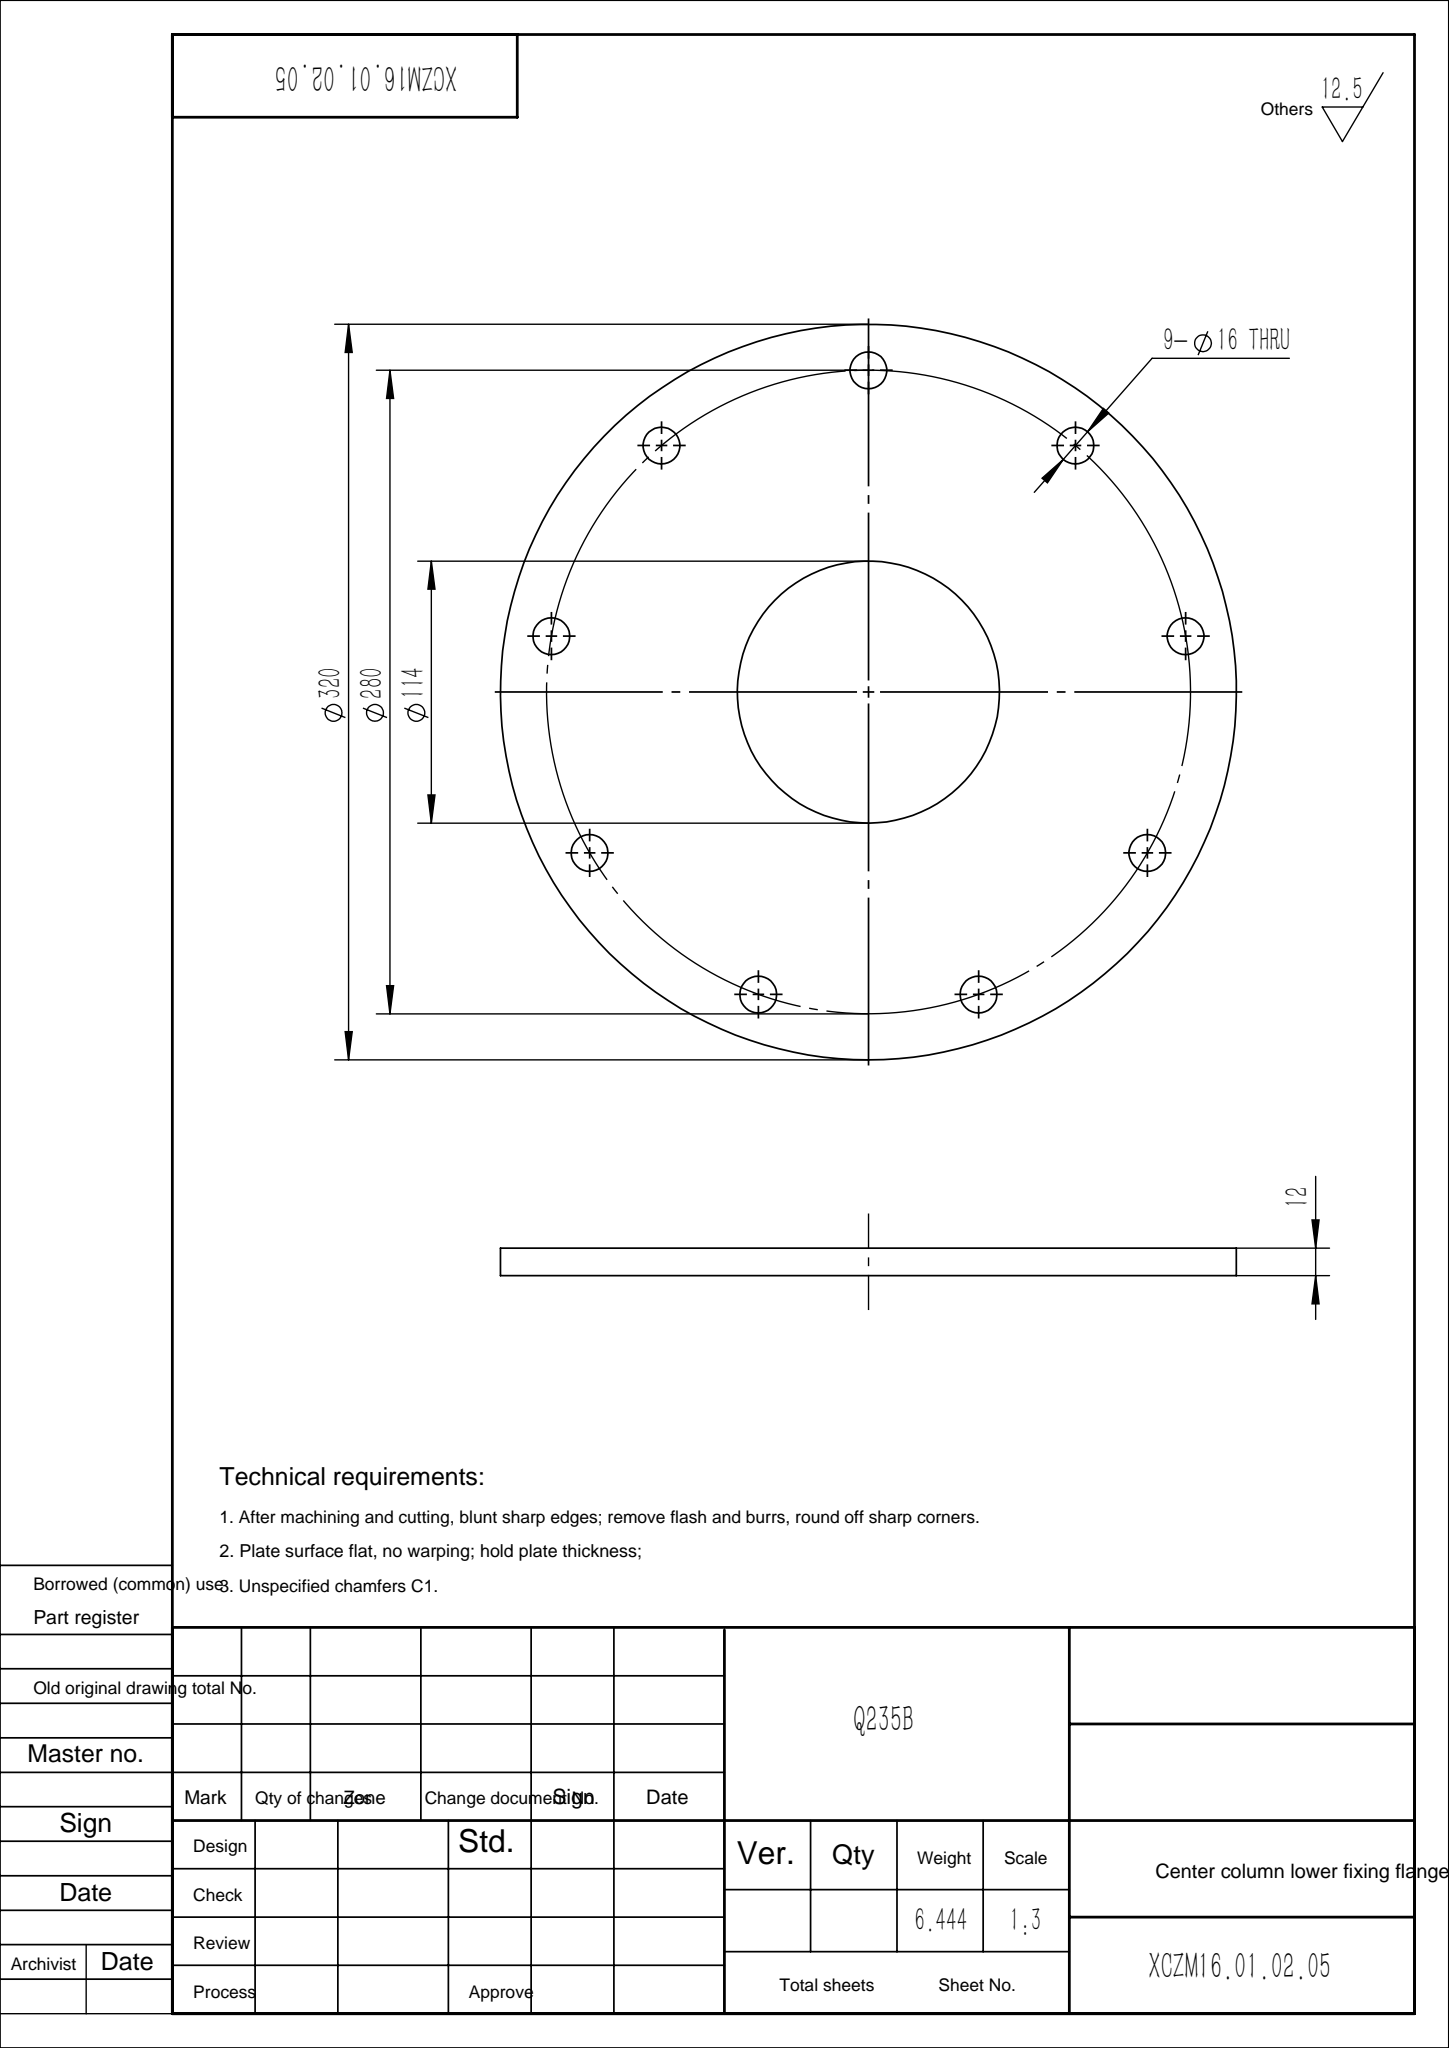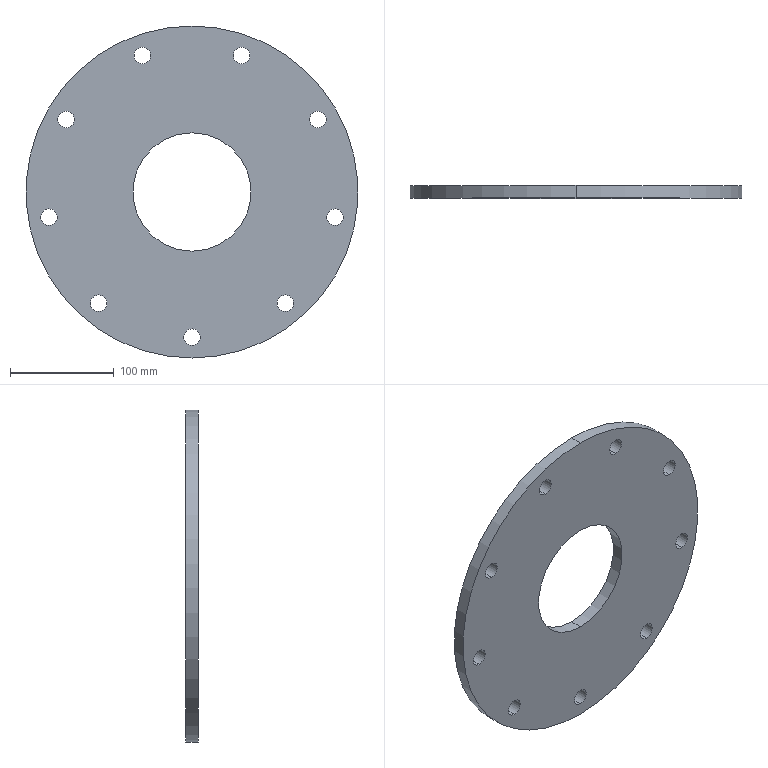Part | SolidWorks | features Extrusion 1 | 1 solid | 24 faces | box 320 x 12 x 320 mm | volume 820898 mm3 | cylinder 22 | plane 2 | commonest cylinder face diameters 16 x18 114 x2 320 x2
STEP:
#1=CARTESIAN_POINT('',(-89.99,12.,-115.246));
#2=VERTEX_POINT('',#1);
#3=CARTESIAN_POINT('',(-89.99,12.,-99.246));
#4=VERTEX_POINT('',#3);
#5=CARTESIAN_POINT('',(-89.99,12.,-107.246));
#6=DIRECTION('',(0.,1.,0.));
#7=DIRECTION('',(0.,0.,1.));
#8=AXIS2_PLACEMENT_3D('',#5,#6,#7);
#9=CIRCLE('',#8,8.);
#10=EDGE_CURVE('',#2,#4,#9,.T.);
#11=ORIENTED_EDGE('',*,*,#10,.T.);
#12=CARTESIAN_POINT('',(-89.99,0.,-99.246));
#13=VERTEX_POINT('',#12);
#14=CARTESIAN_POINT('',(-89.99,12.,-99.246));
#15=DIRECTION('',(0.,-1.,0.));
#16=VECTOR('',#15,1000.);
#17=LINE('',#14,#16);
#18=EDGE_CURVE('',#4,#13,#17,.T.);
#19=ORIENTED_EDGE('',*,*,#18,.T.);
#20=CARTESIAN_POINT('',(-89.99,0.,-115.246));
#21=VERTEX_POINT('',#20);
#22=CARTESIAN_POINT('',(-89.99,0.,-107.246));
#23=DIRECTION('',(0.,1.,0.));
#24=DIRECTION('',(0.,0.,1.));
#25=AXIS2_PLACEMENT_3D('',#22,#23,#24);
#26=CIRCLE('',#25,8.);
#27=EDGE_CURVE('',#21,#13,#26,.T.);
#28=ORIENTED_EDGE('',*,*,#27,.F.);
#29=CARTESIAN_POINT('',(-89.99,12.,-115.246));
#30=DIRECTION('',(0.,-1.,0.));
#31=VECTOR('',#30,1000.);
#32=LINE('',#29,#31);
#33=EDGE_CURVE('',#2,#21,#32,.T.);
#34=ORIENTED_EDGE('',*,*,#33,.F.);
#35=EDGE_LOOP('',(#11,#19,#28,#34));
#36=FACE_OUTER_BOUND('',#35,.T.);
#37=CARTESIAN_POINT('',(-89.99,12.,-107.246));
#38=DIRECTION('',(0.,-1.,0.));
#39=DIRECTION('',(0.,0.,-1.));
#40=AXIS2_PLACEMENT_3D('',#37,#38,#39);
#41=CYLINDRICAL_SURFACE('',#40,8.);
#42=ADVANCED_FACE('',(#36),#41,.F.);
#43=CARTESIAN_POINT('',(-137.873,12.,-32.311));
#44=VERTEX_POINT('',#43);
#45=CARTESIAN_POINT('',(-137.873,12.,-16.311));
#46=VERTEX_POINT('',#45);
#47=CARTESIAN_POINT('',(-137.873,12.,-24.311));
#48=DIRECTION('',(0.,1.,0.));
#49=DIRECTION('',(0.,0.,1.));
#50=AXIS2_PLACEMENT_3D('',#47,#48,#49);
#51=CIRCLE('',#50,8.);
#52=EDGE_CURVE('',#44,#46,#51,.T.);
#53=ORIENTED_EDGE('',*,*,#52,.T.);
#54=CARTESIAN_POINT('',(-137.873,0.,-16.311));
#55=VERTEX_POINT('',#54);
#56=CARTESIAN_POINT('',(-137.873,12.,-16.311));
#57=DIRECTION('',(0.,-1.,0.));
#58=VECTOR('',#57,1000.);
#59=LINE('',#56,#58);
#60=EDGE_CURVE('',#46,#55,#59,.T.);
#61=ORIENTED_EDGE('',*,*,#60,.T.);
#62=CARTESIAN_POINT('',(-137.873,0.,-32.311));
#63=VERTEX_POINT('',#62);
#64=CARTESIAN_POINT('',(-137.873,0.,-24.311));
#65=DIRECTION('',(0.,1.,0.));
#66=DIRECTION('',(0.,0.,1.));
#67=AXIS2_PLACEMENT_3D('',#64,#65,#66);
#68=CIRCLE('',#67,8.);
#69=EDGE_CURVE('',#63,#55,#68,.T.);
#70=ORIENTED_EDGE('',*,*,#69,.F.);
#71=CARTESIAN_POINT('',(-137.873,12.,-32.311));
#72=DIRECTION('',(0.,-1.,0.));
#73=VECTOR('',#72,1000.);
#74=LINE('',#71,#73);
#75=EDGE_CURVE('',#44,#63,#74,.T.);
#76=ORIENTED_EDGE('',*,*,#75,.F.);
#77=EDGE_LOOP('',(#53,#61,#70,#76));
#78=FACE_OUTER_BOUND('',#77,.T.);
#79=CARTESIAN_POINT('',(-137.873,12.,-24.311));
#80=DIRECTION('',(0.,-1.,0.));
#81=DIRECTION('',(0.,0.,-1.));
#82=AXIS2_PLACEMENT_3D('',#79,#80,#81);
#83=CYLINDRICAL_SURFACE('',#82,8.);
#84=ADVANCED_FACE('',(#78),#83,.F.);
#85=CARTESIAN_POINT('',(-121.244,12.,62.));
#86=VERTEX_POINT('',#85);
#87=CARTESIAN_POINT('',(-121.244,12.,78.));
#88=VERTEX_POINT('',#87);
#89=CARTESIAN_POINT('',(-121.244,12.,70.));
#90=DIRECTION('',(0.,1.,0.));
#91=DIRECTION('',(0.,0.,1.));
#92=AXIS2_PLACEMENT_3D('',#89,#90,#91);
#93=CIRCLE('',#92,8.);
#94=EDGE_CURVE('',#86,#88,#93,.T.);
#95=ORIENTED_EDGE('',*,*,#94,.T.);
#96=CARTESIAN_POINT('',(-121.244,0.,78.));
#97=VERTEX_POINT('',#96);
#98=CARTESIAN_POINT('',(-121.244,12.,78.));
#99=DIRECTION('',(0.,-1.,0.));
#100=VECTOR('',#99,1000.);
#101=LINE('',#98,#100);
#102=EDGE_CURVE('',#88,#97,#101,.T.);
#103=ORIENTED_EDGE('',*,*,#102,.T.);
#104=CARTESIAN_POINT('',(-121.244,0.,62.));
#105=VERTEX_POINT('',#104);
#106=CARTESIAN_POINT('',(-121.244,0.,70.));
#107=DIRECTION('',(0.,1.,0.));
#108=DIRECTION('',(0.,0.,1.));
#109=AXIS2_PLACEMENT_3D('',#106,#107,#108);
#110=CIRCLE('',#109,8.);
#111=EDGE_CURVE('',#105,#97,#110,.T.);
#112=ORIENTED_EDGE('',*,*,#111,.F.);
#113=CARTESIAN_POINT('',(-121.244,12.,62.));
#114=DIRECTION('',(0.,-1.,0.));
#115=VECTOR('',#114,1000.);
#116=LINE('',#113,#115);
#117=EDGE_CURVE('',#86,#105,#116,.T.);
#118=ORIENTED_EDGE('',*,*,#117,.F.);
#119=EDGE_LOOP('',(#95,#103,#112,#118));
#120=FACE_OUTER_BOUND('',#119,.T.);
#121=CARTESIAN_POINT('',(-121.244,12.,70.));
#122=DIRECTION('',(0.,-1.,0.));
#123=DIRECTION('',(0.,0.,-1.));
#124=AXIS2_PLACEMENT_3D('',#121,#122,#123);
#125=CYLINDRICAL_SURFACE('',#124,8.);
#126=ADVANCED_FACE('',(#120),#125,.F.);
#127=CARTESIAN_POINT('',(-47.883,12.,123.557));
#128=VERTEX_POINT('',#127);
#129=CARTESIAN_POINT('',(-47.883,12.,139.557));
#130=VERTEX_POINT('',#129);
#131=CARTESIAN_POINT('',(-47.883,12.,131.557));
#132=DIRECTION('',(0.,1.,0.));
#133=DIRECTION('',(0.,0.,1.));
#134=AXIS2_PLACEMENT_3D('',#131,#132,#133);
#135=CIRCLE('',#134,8.);
#136=EDGE_CURVE('',#128,#130,#135,.T.);
#137=ORIENTED_EDGE('',*,*,#136,.T.);
#138=CARTESIAN_POINT('',(-47.883,0.,139.557));
#139=VERTEX_POINT('',#138);
#140=CARTESIAN_POINT('',(-47.883,12.,139.557));
#141=DIRECTION('',(0.,-1.,0.));
#142=VECTOR('',#141,1000.);
#143=LINE('',#140,#142);
#144=EDGE_CURVE('',#130,#139,#143,.T.);
#145=ORIENTED_EDGE('',*,*,#144,.T.);
#146=CARTESIAN_POINT('',(-47.883,0.,123.557));
#147=VERTEX_POINT('',#146);
#148=CARTESIAN_POINT('',(-47.883,0.,131.557));
#149=DIRECTION('',(0.,1.,0.));
#150=DIRECTION('',(0.,0.,1.));
#151=AXIS2_PLACEMENT_3D('',#148,#149,#150);
#152=CIRCLE('',#151,8.);
#153=EDGE_CURVE('',#147,#139,#152,.T.);
#154=ORIENTED_EDGE('',*,*,#153,.F.);
#155=CARTESIAN_POINT('',(-47.883,12.,123.557));
#156=DIRECTION('',(0.,-1.,0.));
#157=VECTOR('',#156,1000.);
#158=LINE('',#155,#157);
#159=EDGE_CURVE('',#128,#147,#158,.T.);
#160=ORIENTED_EDGE('',*,*,#159,.F.);
#161=EDGE_LOOP('',(#137,#145,#154,#160));
#162=FACE_OUTER_BOUND('',#161,.T.);
#163=CARTESIAN_POINT('',(-47.883,12.,131.557));
#164=DIRECTION('',(0.,-1.,0.));
#165=DIRECTION('',(0.,0.,-1.));
#166=AXIS2_PLACEMENT_3D('',#163,#164,#165);
#167=CYLINDRICAL_SURFACE('',#166,8.);
#168=ADVANCED_FACE('',(#162),#167,.F.);
#169=CARTESIAN_POINT('',(47.883,12.,123.557));
#170=VERTEX_POINT('',#169);
#171=CARTESIAN_POINT('',(47.883,12.,139.557));
#172=VERTEX_POINT('',#171);
#173=CARTESIAN_POINT('',(47.883,12.,131.557));
#174=DIRECTION('',(0.,1.,0.));
#175=DIRECTION('',(0.,0.,1.));
#176=AXIS2_PLACEMENT_3D('',#173,#174,#175);
#177=CIRCLE('',#176,8.);
#178=EDGE_CURVE('',#170,#172,#177,.T.);
#179=ORIENTED_EDGE('',*,*,#178,.T.);
#180=CARTESIAN_POINT('',(47.883,0.,139.557));
#181=VERTEX_POINT('',#180);
#182=CARTESIAN_POINT('',(47.883,12.,139.557));
#183=DIRECTION('',(0.,-1.,0.));
#184=VECTOR('',#183,1000.);
#185=LINE('',#182,#184);
#186=EDGE_CURVE('',#172,#181,#185,.T.);
#187=ORIENTED_EDGE('',*,*,#186,.T.);
#188=CARTESIAN_POINT('',(47.883,0.,123.557));
#189=VERTEX_POINT('',#188);
#190=CARTESIAN_POINT('',(47.883,0.,131.557));
#191=DIRECTION('',(0.,1.,0.));
#192=DIRECTION('',(0.,0.,1.));
#193=AXIS2_PLACEMENT_3D('',#190,#191,#192);
#194=CIRCLE('',#193,8.);
#195=EDGE_CURVE('',#189,#181,#194,.T.);
#196=ORIENTED_EDGE('',*,*,#195,.F.);
#197=CARTESIAN_POINT('',(47.883,12.,123.557));
#198=DIRECTION('',(0.,-1.,0.));
#199=VECTOR('',#198,1000.);
#200=LINE('',#197,#199);
#201=EDGE_CURVE('',#170,#189,#200,.T.);
#202=ORIENTED_EDGE('',*,*,#201,.F.);
#203=EDGE_LOOP('',(#179,#187,#196,#202));
#204=FACE_OUTER_BOUND('',#203,.T.);
#205=CARTESIAN_POINT('',(47.883,12.,131.557));
#206=DIRECTION('',(0.,-1.,0.));
#207=DIRECTION('',(0.,0.,-1.));
#208=AXIS2_PLACEMENT_3D('',#205,#206,#207);
#209=CYLINDRICAL_SURFACE('',#208,8.);
#210=ADVANCED_FACE('',(#204),#209,.F.);
#211=CARTESIAN_POINT('',(121.244,12.,62.));
#212=VERTEX_POINT('',#211);
#213=CARTESIAN_POINT('',(121.244,12.,78.));
#214=VERTEX_POINT('',#213);
#215=CARTESIAN_POINT('',(121.244,12.,70.));
#216=DIRECTION('',(0.,1.,0.));
#217=DIRECTION('',(0.,0.,1.));
#218=AXIS2_PLACEMENT_3D('',#215,#216,#217);
#219=CIRCLE('',#218,8.);
#220=EDGE_CURVE('',#212,#214,#219,.T.);
#221=ORIENTED_EDGE('',*,*,#220,.T.);
#222=CARTESIAN_POINT('',(121.244,0.,78.));
#223=VERTEX_POINT('',#222);
#224=CARTESIAN_POINT('',(121.244,12.,78.));
#225=DIRECTION('',(0.,-1.,0.));
#226=VECTOR('',#225,1000.);
#227=LINE('',#224,#226);
#228=EDGE_CURVE('',#214,#223,#227,.T.);
#229=ORIENTED_EDGE('',*,*,#228,.T.);
#230=CARTESIAN_POINT('',(121.244,0.,62.));
#231=VERTEX_POINT('',#230);
#232=CARTESIAN_POINT('',(121.244,0.,70.));
#233=DIRECTION('',(0.,1.,0.));
#234=DIRECTION('',(0.,0.,1.));
#235=AXIS2_PLACEMENT_3D('',#232,#233,#234);
#236=CIRCLE('',#235,8.);
#237=EDGE_CURVE('',#231,#223,#236,.T.);
#238=ORIENTED_EDGE('',*,*,#237,.F.);
#239=CARTESIAN_POINT('',(121.244,12.,62.));
#240=DIRECTION('',(0.,-1.,0.));
#241=VECTOR('',#240,1000.);
#242=LINE('',#239,#241);
#243=EDGE_CURVE('',#212,#231,#242,.T.);
#244=ORIENTED_EDGE('',*,*,#243,.F.);
#245=EDGE_LOOP('',(#221,#229,#238,#244));
#246=FACE_OUTER_BOUND('',#245,.T.);
#247=CARTESIAN_POINT('',(121.244,12.,70.));
#248=DIRECTION('',(0.,-1.,0.));
#249=DIRECTION('',(0.,0.,-1.));
#250=AXIS2_PLACEMENT_3D('',#247,#248,#249);
#251=CYLINDRICAL_SURFACE('',#250,8.);
#252=ADVANCED_FACE('',(#246),#251,.F.);
#253=CARTESIAN_POINT('',(137.873,12.,-32.311));
#254=VERTEX_POINT('',#253);
#255=CARTESIAN_POINT('',(137.873,12.,-16.311));
#256=VERTEX_POINT('',#255);
#257=CARTESIAN_POINT('',(137.873,12.,-24.311));
#258=DIRECTION('',(0.,1.,0.));
#259=DIRECTION('',(0.,0.,1.));
#260=AXIS2_PLACEMENT_3D('',#257,#258,#259);
#261=CIRCLE('',#260,8.);
#262=EDGE_CURVE('',#254,#256,#261,.T.);
#263=ORIENTED_EDGE('',*,*,#262,.T.);
#264=CARTESIAN_POINT('',(137.873,0.,-16.311));
#265=VERTEX_POINT('',#264);
#266=CARTESIAN_POINT('',(137.873,12.,-16.311));
#267=DIRECTION('',(0.,-1.,0.));
#268=VECTOR('',#267,1000.);
#269=LINE('',#266,#268);
#270=EDGE_CURVE('',#256,#265,#269,.T.);
#271=ORIENTED_EDGE('',*,*,#270,.T.);
#272=CARTESIAN_POINT('',(137.873,0.,-32.311));
#273=VERTEX_POINT('',#272);
#274=CARTESIAN_POINT('',(137.873,0.,-24.311));
#275=DIRECTION('',(0.,1.,0.));
#276=DIRECTION('',(0.,0.,1.));
#277=AXIS2_PLACEMENT_3D('',#274,#275,#276);
#278=CIRCLE('',#277,8.);
#279=EDGE_CURVE('',#273,#265,#278,.T.);
#280=ORIENTED_EDGE('',*,*,#279,.F.);
#281=CARTESIAN_POINT('',(137.873,12.,-32.311));
#282=DIRECTION('',(0.,-1.,0.));
#283=VECTOR('',#282,1000.);
#284=LINE('',#281,#283);
#285=EDGE_CURVE('',#254,#273,#284,.T.);
#286=ORIENTED_EDGE('',*,*,#285,.F.);
#287=EDGE_LOOP('',(#263,#271,#280,#286));
#288=FACE_OUTER_BOUND('',#287,.T.);
#289=CARTESIAN_POINT('',(137.873,12.,-24.311));
#290=DIRECTION('',(0.,-1.,0.));
#291=DIRECTION('',(0.,0.,-1.));
#292=AXIS2_PLACEMENT_3D('',#289,#290,#291);
#293=CYLINDRICAL_SURFACE('',#292,8.);
#294=ADVANCED_FACE('',(#288),#293,.F.);
#295=CARTESIAN_POINT('',(89.99,12.,-115.246));
#296=VERTEX_POINT('',#295);
#297=CARTESIAN_POINT('',(89.99,12.,-99.246));
#298=VERTEX_POINT('',#297);
#299=CARTESIAN_POINT('',(89.99,12.,-107.246));
#300=DIRECTION('',(0.,1.,0.));
#301=DIRECTION('',(0.,0.,1.));
#302=AXIS2_PLACEMENT_3D('',#299,#300,#301);
#303=CIRCLE('',#302,8.);
#304=EDGE_CURVE('',#296,#298,#303,.T.);
#305=ORIENTED_EDGE('',*,*,#304,.T.);
#306=CARTESIAN_POINT('',(89.99,0.,-99.246));
#307=VERTEX_POINT('',#306);
#308=CARTESIAN_POINT('',(89.99,12.,-99.246));
#309=DIRECTION('',(0.,-1.,0.));
#310=VECTOR('',#309,1000.);
#311=LINE('',#308,#310);
#312=EDGE_CURVE('',#298,#307,#311,.T.);
#313=ORIENTED_EDGE('',*,*,#312,.T.);
#314=CARTESIAN_POINT('',(89.99,0.,-115.246));
#315=VERTEX_POINT('',#314);
#316=CARTESIAN_POINT('',(89.99,0.,-107.246));
#317=DIRECTION('',(0.,1.,0.));
#318=DIRECTION('',(0.,0.,1.));
#319=AXIS2_PLACEMENT_3D('',#316,#317,#318);
#320=CIRCLE('',#319,8.);
#321=EDGE_CURVE('',#315,#307,#320,.T.);
#322=ORIENTED_EDGE('',*,*,#321,.F.);
#323=CARTESIAN_POINT('',(89.99,12.,-115.246));
#324=DIRECTION('',(0.,-1.,0.));
#325=VECTOR('',#324,1000.);
#326=LINE('',#323,#325);
#327=EDGE_CURVE('',#296,#315,#326,.T.);
#328=ORIENTED_EDGE('',*,*,#327,.F.);
#329=EDGE_LOOP('',(#305,#313,#322,#328));
#330=FACE_OUTER_BOUND('',#329,.T.);
#331=CARTESIAN_POINT('',(89.99,12.,-107.246));
#332=DIRECTION('',(0.,-1.,0.));
#333=DIRECTION('',(0.,0.,-1.));
#334=AXIS2_PLACEMENT_3D('',#331,#332,#333);
#335=CYLINDRICAL_SURFACE('',#334,8.);
#336=ADVANCED_FACE('',(#330),#335,.F.);
#337=CARTESIAN_POINT('',(0.,12.,-148.));
#338=VERTEX_POINT('',#337);
#339=CARTESIAN_POINT('',(0.,12.,-132.));
#340=VERTEX_POINT('',#339);
#341=CARTESIAN_POINT('',(0.,12.,-140.));
#342=DIRECTION('',(0.,1.,0.));
#343=DIRECTION('',(0.,0.,1.));
#344=AXIS2_PLACEMENT_3D('',#341,#342,#343);
#345=CIRCLE('',#344,8.);
#346=EDGE_CURVE('',#338,#340,#345,.T.);
#347=ORIENTED_EDGE('',*,*,#346,.T.);
#348=CARTESIAN_POINT('',(0.,0.,-132.));
#349=VERTEX_POINT('',#348);
#350=CARTESIAN_POINT('',(0.,12.,-132.));
#351=DIRECTION('',(0.,-1.,0.));
#352=VECTOR('',#351,1000.);
#353=LINE('',#350,#352);
#354=EDGE_CURVE('',#340,#349,#353,.T.);
#355=ORIENTED_EDGE('',*,*,#354,.T.);
#356=CARTESIAN_POINT('',(0.,0.,-148.));
#357=VERTEX_POINT('',#356);
#358=CARTESIAN_POINT('',(0.,0.,-140.));
#359=DIRECTION('',(0.,1.,0.));
#360=DIRECTION('',(0.,0.,1.));
#361=AXIS2_PLACEMENT_3D('',#358,#359,#360);
#362=CIRCLE('',#361,8.);
#363=EDGE_CURVE('',#357,#349,#362,.T.);
#364=ORIENTED_EDGE('',*,*,#363,.F.);
#365=CARTESIAN_POINT('',(0.,12.,-148.));
#366=DIRECTION('',(0.,-1.,0.));
#367=VECTOR('',#366,1000.);
#368=LINE('',#365,#367);
#369=EDGE_CURVE('',#338,#357,#368,.T.);
#370=ORIENTED_EDGE('',*,*,#369,.F.);
#371=EDGE_LOOP('',(#347,#355,#364,#370));
#372=FACE_OUTER_BOUND('',#371,.T.);
#373=CARTESIAN_POINT('',(0.,12.,-140.));
#374=DIRECTION('',(0.,-1.,0.));
#375=DIRECTION('',(0.,0.,-1.));
#376=AXIS2_PLACEMENT_3D('',#373,#374,#375);
#377=CYLINDRICAL_SURFACE('',#376,8.);
#378=ADVANCED_FACE('',(#372),#377,.F.);
#379=CARTESIAN_POINT('',(0.,12.,-57.));
#380=VERTEX_POINT('',#379);
#381=CARTESIAN_POINT('',(0.,12.,57.));
#382=VERTEX_POINT('',#381);
#383=CARTESIAN_POINT('',(0.,12.,0.));
#384=DIRECTION('',(0.,1.,0.));
#385=DIRECTION('',(0.,0.,1.));
#386=AXIS2_PLACEMENT_3D('',#383,#384,#385);
#387=CIRCLE('',#386,57.);
#388=EDGE_CURVE('',#380,#382,#387,.T.);
#389=ORIENTED_EDGE('',*,*,#388,.T.);
#390=CARTESIAN_POINT('',(0.,0.,57.));
#391=VERTEX_POINT('',#390);
#392=CARTESIAN_POINT('',(0.,12.,57.));
#393=DIRECTION('',(0.,-1.,0.));
#394=VECTOR('',#393,1000.);
#395=LINE('',#392,#394);
#396=EDGE_CURVE('',#382,#391,#395,.T.);
#397=ORIENTED_EDGE('',*,*,#396,.T.);
#398=CARTESIAN_POINT('',(0.,0.,-57.));
#399=VERTEX_POINT('',#398);
#400=CARTESIAN_POINT('',(0.,0.,0.));
#401=DIRECTION('',(0.,1.,0.));
#402=DIRECTION('',(0.,0.,1.));
#403=AXIS2_PLACEMENT_3D('',#400,#401,#402);
#404=CIRCLE('',#403,57.);
#405=EDGE_CURVE('',#399,#391,#404,.T.);
#406=ORIENTED_EDGE('',*,*,#405,.F.);
#407=CARTESIAN_POINT('',(0.,12.,-57.));
#408=DIRECTION('',(0.,-1.,0.));
#409=VECTOR('',#408,1000.);
#410=LINE('',#407,#409);
#411=EDGE_CURVE('',#380,#399,#410,.T.);
#412=ORIENTED_EDGE('',*,*,#411,.F.);
#413=EDGE_LOOP('',(#389,#397,#406,#412));
#414=FACE_OUTER_BOUND('',#413,.T.);
#415=CARTESIAN_POINT('',(0.,12.,0.));
#416=DIRECTION('',(0.,-1.,0.));
#417=DIRECTION('',(0.,0.,-1.));
#418=AXIS2_PLACEMENT_3D('',#415,#416,#417);
#419=CYLINDRICAL_SURFACE('',#418,57.);
#420=ADVANCED_FACE('',(#414),#419,.F.);
#421=CARTESIAN_POINT('',(0.,12.,160.));
#422=VERTEX_POINT('',#421);
#423=CARTESIAN_POINT('',(0.,12.,-160.));
#424=VERTEX_POINT('',#423);
#425=CARTESIAN_POINT('',(0.,12.,0.));
#426=DIRECTION('',(0.,1.,0.));
#427=DIRECTION('',(0.,0.,1.));
#428=AXIS2_PLACEMENT_3D('',#425,#426,#427);
#429=CIRCLE('',#428,160.);
#430=EDGE_CURVE('',#422,#424,#429,.T.);
#431=ORIENTED_EDGE('',*,*,#430,.F.);
#432=CARTESIAN_POINT('',(0.,0.,160.));
#433=VERTEX_POINT('',#432);
#434=CARTESIAN_POINT('',(0.,12.,160.));
#435=DIRECTION('',(0.,-1.,0.));
#436=VECTOR('',#435,1000.);
#437=LINE('',#434,#436);
#438=EDGE_CURVE('',#422,#433,#437,.T.);
#439=ORIENTED_EDGE('',*,*,#438,.T.);
#440=CARTESIAN_POINT('',(0.,0.,-160.));
#441=VERTEX_POINT('',#440);
#442=CARTESIAN_POINT('',(0.,0.,0.));
#443=DIRECTION('',(0.,1.,0.));
#444=DIRECTION('',(0.,0.,1.));
#445=AXIS2_PLACEMENT_3D('',#442,#443,#444);
#446=CIRCLE('',#445,160.);
#447=EDGE_CURVE('',#433,#441,#446,.T.);
#448=ORIENTED_EDGE('',*,*,#447,.T.);
#449=CARTESIAN_POINT('',(0.,12.,-160.));
#450=DIRECTION('',(0.,-1.,0.));
#451=VECTOR('',#450,1000.);
#452=LINE('',#449,#451);
#453=EDGE_CURVE('',#424,#441,#452,.T.);
#454=ORIENTED_EDGE('',*,*,#453,.F.);
#455=EDGE_LOOP('',(#431,#439,#448,#454));
#456=FACE_OUTER_BOUND('',#455,.T.);
#457=CARTESIAN_POINT('',(0.,12.,0.));
#458=DIRECTION('',(0.,-1.,0.));
#459=DIRECTION('',(0.,0.,-1.));
#460=AXIS2_PLACEMENT_3D('',#457,#458,#459);
#461=CYLINDRICAL_SURFACE('',#460,160.);
#462=ADVANCED_FACE('',(#456),#461,.T.);
#463=ORIENTED_EDGE('',*,*,#52,.F.);
#464=CARTESIAN_POINT('',(-137.873,12.,-24.311));
#465=DIRECTION('',(0.,1.,0.));
#466=DIRECTION('',(0.,0.,1.));
#467=AXIS2_PLACEMENT_3D('',#464,#465,#466);
#468=CIRCLE('',#467,8.);
#469=EDGE_CURVE('',#46,#44,#468,.T.);
#470=ORIENTED_EDGE('',*,*,#469,.F.);
#471=EDGE_LOOP('',(#463,#470));
#472=FACE_BOUND('',#471,.T.);
#473=ORIENTED_EDGE('',*,*,#136,.F.);
#474=CARTESIAN_POINT('',(-47.883,12.,131.557));
#475=DIRECTION('',(0.,1.,0.));
#476=DIRECTION('',(0.,0.,1.));
#477=AXIS2_PLACEMENT_3D('',#474,#475,#476);
#478=CIRCLE('',#477,8.);
#479=EDGE_CURVE('',#130,#128,#478,.T.);
#480=ORIENTED_EDGE('',*,*,#479,.F.);
#481=EDGE_LOOP('',(#473,#480));
#482=FACE_BOUND('',#481,.T.);
#483=ORIENTED_EDGE('',*,*,#220,.F.);
#484=CARTESIAN_POINT('',(121.244,12.,70.));
#485=DIRECTION('',(0.,1.,0.));
#486=DIRECTION('',(0.,0.,1.));
#487=AXIS2_PLACEMENT_3D('',#484,#485,#486);
#488=CIRCLE('',#487,8.);
#489=EDGE_CURVE('',#214,#212,#488,.T.);
#490=ORIENTED_EDGE('',*,*,#489,.F.);
#491=EDGE_LOOP('',(#483,#490));
#492=FACE_BOUND('',#491,.T.);
#493=ORIENTED_EDGE('',*,*,#304,.F.);
#494=CARTESIAN_POINT('',(89.99,12.,-107.246));
#495=DIRECTION('',(0.,1.,0.));
#496=DIRECTION('',(0.,0.,1.));
#497=AXIS2_PLACEMENT_3D('',#494,#495,#496);
#498=CIRCLE('',#497,8.);
#499=EDGE_CURVE('',#298,#296,#498,.T.);
#500=ORIENTED_EDGE('',*,*,#499,.F.);
#501=EDGE_LOOP('',(#493,#500));
#502=FACE_BOUND('',#501,.T.);
#503=ORIENTED_EDGE('',*,*,#388,.F.);
#504=CARTESIAN_POINT('',(0.,12.,0.));
#505=DIRECTION('',(0.,1.,0.));
#506=DIRECTION('',(0.,0.,1.));
#507=AXIS2_PLACEMENT_3D('',#504,#505,#506);
#508=CIRCLE('',#507,57.);
#509=EDGE_CURVE('',#382,#380,#508,.T.);
#510=ORIENTED_EDGE('',*,*,#509,.F.);
#511=EDGE_LOOP('',(#503,#510));
#512=FACE_BOUND('',#511,.T.);
#513=CARTESIAN_POINT('',(0.,12.,0.));
#514=DIRECTION('',(0.,1.,0.));
#515=DIRECTION('',(0.,0.,1.));
#516=AXIS2_PLACEMENT_3D('',#513,#514,#515);
#517=CIRCLE('',#516,160.);
#518=EDGE_CURVE('',#424,#422,#517,.T.);
#519=ORIENTED_EDGE('',*,*,#518,.T.);
#520=ORIENTED_EDGE('',*,*,#430,.T.);
#521=EDGE_LOOP('',(#519,#520));
#522=FACE_OUTER_BOUND('',#521,.T.);
#523=ORIENTED_EDGE('',*,*,#346,.F.);
#524=CARTESIAN_POINT('',(0.,12.,-140.));
#525=DIRECTION('',(0.,1.,0.));
#526=DIRECTION('',(0.,0.,1.));
#527=AXIS2_PLACEMENT_3D('',#524,#525,#526);
#528=CIRCLE('',#527,8.);
#529=EDGE_CURVE('',#340,#338,#528,.T.);
#530=ORIENTED_EDGE('',*,*,#529,.F.);
#531=EDGE_LOOP('',(#523,#530));
#532=FACE_BOUND('',#531,.T.);
#533=ORIENTED_EDGE('',*,*,#262,.F.);
#534=CARTESIAN_POINT('',(137.873,12.,-24.311));
#535=DIRECTION('',(0.,1.,0.));
#536=DIRECTION('',(0.,0.,1.));
#537=AXIS2_PLACEMENT_3D('',#534,#535,#536);
#538=CIRCLE('',#537,8.);
#539=EDGE_CURVE('',#256,#254,#538,.T.);
#540=ORIENTED_EDGE('',*,*,#539,.F.);
#541=EDGE_LOOP('',(#533,#540));
#542=FACE_BOUND('',#541,.T.);
#543=ORIENTED_EDGE('',*,*,#178,.F.);
#544=CARTESIAN_POINT('',(47.883,12.,131.557));
#545=DIRECTION('',(0.,1.,0.));
#546=DIRECTION('',(0.,0.,1.));
#547=AXIS2_PLACEMENT_3D('',#544,#545,#546);
#548=CIRCLE('',#547,8.);
#549=EDGE_CURVE('',#172,#170,#548,.T.);
#550=ORIENTED_EDGE('',*,*,#549,.F.);
#551=EDGE_LOOP('',(#543,#550));
#552=FACE_BOUND('',#551,.T.);
#553=ORIENTED_EDGE('',*,*,#94,.F.);
#554=CARTESIAN_POINT('',(-121.244,12.,70.));
#555=DIRECTION('',(0.,1.,0.));
#556=DIRECTION('',(0.,0.,1.));
#557=AXIS2_PLACEMENT_3D('',#554,#555,#556);
#558=CIRCLE('',#557,8.);
#559=EDGE_CURVE('',#88,#86,#558,.T.);
#560=ORIENTED_EDGE('',*,*,#559,.F.);
#561=EDGE_LOOP('',(#553,#560));
#562=FACE_BOUND('',#561,.T.);
#563=ORIENTED_EDGE('',*,*,#10,.F.);
#564=CARTESIAN_POINT('',(-89.99,12.,-107.246));
#565=DIRECTION('',(0.,1.,0.));
#566=DIRECTION('',(0.,0.,1.));
#567=AXIS2_PLACEMENT_3D('',#564,#565,#566);
#568=CIRCLE('',#567,8.);
#569=EDGE_CURVE('',#4,#2,#568,.T.);
#570=ORIENTED_EDGE('',*,*,#569,.F.);
#571=EDGE_LOOP('',(#563,#570));
#572=FACE_BOUND('',#571,.T.);
#573=CARTESIAN_POINT('',(0.,12.,0.));
#574=DIRECTION('',(0.,1.,0.));
#575=DIRECTION('',(0.,0.,1.));
#576=AXIS2_PLACEMENT_3D('',#573,#574,#575);
#577=PLANE('',#576);
#578=ADVANCED_FACE('',(#472,#482,#492,#502,#512,#522,#532,#542,#552,#562,#572),#577,.T.);
#579=CARTESIAN_POINT('',(0.,0.,0.));
#580=DIRECTION('',(0.,1.,0.));
#581=DIRECTION('',(0.,0.,1.));
#582=AXIS2_PLACEMENT_3D('',#579,#580,#581);
#583=CIRCLE('',#582,160.);
#584=EDGE_CURVE('',#441,#433,#583,.T.);
#585=ORIENTED_EDGE('',*,*,#584,.F.);
#586=ORIENTED_EDGE('',*,*,#447,.F.);
#587=EDGE_LOOP('',(#585,#586));
#588=FACE_OUTER_BOUND('',#587,.T.);
#589=ORIENTED_EDGE('',*,*,#405,.T.);
#590=CARTESIAN_POINT('',(0.,0.,0.));
#591=DIRECTION('',(0.,1.,0.));
#592=DIRECTION('',(0.,0.,1.));
#593=AXIS2_PLACEMENT_3D('',#590,#591,#592);
#594=CIRCLE('',#593,57.);
#595=EDGE_CURVE('',#391,#399,#594,.T.);
#596=ORIENTED_EDGE('',*,*,#595,.T.);
#597=EDGE_LOOP('',(#589,#596));
#598=FACE_BOUND('',#597,.T.);
#599=ORIENTED_EDGE('',*,*,#363,.T.);
#600=CARTESIAN_POINT('',(0.,0.,-140.));
#601=DIRECTION('',(0.,1.,0.));
#602=DIRECTION('',(0.,0.,1.));
#603=AXIS2_PLACEMENT_3D('',#600,#601,#602);
#604=CIRCLE('',#603,8.);
#605=EDGE_CURVE('',#349,#357,#604,.T.);
#606=ORIENTED_EDGE('',*,*,#605,.T.);
#607=EDGE_LOOP('',(#599,#606));
#608=FACE_BOUND('',#607,.T.);
#609=ORIENTED_EDGE('',*,*,#321,.T.);
#610=CARTESIAN_POINT('',(89.99,0.,-107.246));
#611=DIRECTION('',(0.,1.,0.));
#612=DIRECTION('',(0.,0.,1.));
#613=AXIS2_PLACEMENT_3D('',#610,#611,#612);
#614=CIRCLE('',#613,8.);
#615=EDGE_CURVE('',#307,#315,#614,.T.);
#616=ORIENTED_EDGE('',*,*,#615,.T.);
#617=EDGE_LOOP('',(#609,#616));
#618=FACE_BOUND('',#617,.T.);
#619=ORIENTED_EDGE('',*,*,#279,.T.);
#620=CARTESIAN_POINT('',(137.873,0.,-24.311));
#621=DIRECTION('',(0.,1.,0.));
#622=DIRECTION('',(0.,0.,1.));
#623=AXIS2_PLACEMENT_3D('',#620,#621,#622);
#624=CIRCLE('',#623,8.);
#625=EDGE_CURVE('',#265,#273,#624,.T.);
#626=ORIENTED_EDGE('',*,*,#625,.T.);
#627=EDGE_LOOP('',(#619,#626));
#628=FACE_BOUND('',#627,.T.);
#629=ORIENTED_EDGE('',*,*,#237,.T.);
#630=CARTESIAN_POINT('',(121.244,0.,70.));
#631=DIRECTION('',(0.,1.,0.));
#632=DIRECTION('',(0.,0.,1.));
#633=AXIS2_PLACEMENT_3D('',#630,#631,#632);
#634=CIRCLE('',#633,8.);
#635=EDGE_CURVE('',#223,#231,#634,.T.);
#636=ORIENTED_EDGE('',*,*,#635,.T.);
#637=EDGE_LOOP('',(#629,#636));
#638=FACE_BOUND('',#637,.T.);
#639=ORIENTED_EDGE('',*,*,#195,.T.);
#640=CARTESIAN_POINT('',(47.883,0.,131.557));
#641=DIRECTION('',(0.,1.,0.));
#642=DIRECTION('',(0.,0.,1.));
#643=AXIS2_PLACEMENT_3D('',#640,#641,#642);
#644=CIRCLE('',#643,8.);
#645=EDGE_CURVE('',#181,#189,#644,.T.);
#646=ORIENTED_EDGE('',*,*,#645,.T.);
#647=EDGE_LOOP('',(#639,#646));
#648=FACE_BOUND('',#647,.T.);
#649=ORIENTED_EDGE('',*,*,#153,.T.);
#650=CARTESIAN_POINT('',(-47.883,0.,131.557));
#651=DIRECTION('',(0.,1.,0.));
#652=DIRECTION('',(0.,0.,1.));
#653=AXIS2_PLACEMENT_3D('',#650,#651,#652);
#654=CIRCLE('',#653,8.);
#655=EDGE_CURVE('',#139,#147,#654,.T.);
#656=ORIENTED_EDGE('',*,*,#655,.T.);
#657=EDGE_LOOP('',(#649,#656));
#658=FACE_BOUND('',#657,.T.);
#659=ORIENTED_EDGE('',*,*,#111,.T.);
#660=CARTESIAN_POINT('',(-121.244,0.,70.));
#661=DIRECTION('',(0.,1.,0.));
#662=DIRECTION('',(0.,0.,1.));
#663=AXIS2_PLACEMENT_3D('',#660,#661,#662);
#664=CIRCLE('',#663,8.);
#665=EDGE_CURVE('',#97,#105,#664,.T.);
#666=ORIENTED_EDGE('',*,*,#665,.T.);
#667=EDGE_LOOP('',(#659,#666));
#668=FACE_BOUND('',#667,.T.);
#669=ORIENTED_EDGE('',*,*,#69,.T.);
#670=CARTESIAN_POINT('',(-137.873,0.,-24.311));
#671=DIRECTION('',(0.,1.,0.));
#672=DIRECTION('',(0.,0.,1.));
#673=AXIS2_PLACEMENT_3D('',#670,#671,#672);
#674=CIRCLE('',#673,8.);
#675=EDGE_CURVE('',#55,#63,#674,.T.);
#676=ORIENTED_EDGE('',*,*,#675,.T.);
#677=EDGE_LOOP('',(#669,#676));
#678=FACE_BOUND('',#677,.T.);
#679=ORIENTED_EDGE('',*,*,#27,.T.);
#680=CARTESIAN_POINT('',(-89.99,0.,-107.246));
#681=DIRECTION('',(0.,1.,0.));
#682=DIRECTION('',(0.,0.,1.));
#683=AXIS2_PLACEMENT_3D('',#680,#681,#682);
#684=CIRCLE('',#683,8.);
#685=EDGE_CURVE('',#13,#21,#684,.T.);
#686=ORIENTED_EDGE('',*,*,#685,.T.);
#687=EDGE_LOOP('',(#679,#686));
#688=FACE_BOUND('',#687,.T.);
#689=CARTESIAN_POINT('',(0.,0.,0.));
#690=DIRECTION('',(0.,1.,0.));
#691=DIRECTION('',(0.,0.,1.));
#692=AXIS2_PLACEMENT_3D('',#689,#690,#691);
#693=PLANE('',#692);
#694=ADVANCED_FACE('',(#588,#598,#608,#618,#628,#638,#648,#658,#668,#678,#688),#693,.F.);
#695=ORIENTED_EDGE('',*,*,#438,.F.);
#696=ORIENTED_EDGE('',*,*,#518,.F.);
#697=ORIENTED_EDGE('',*,*,#453,.T.);
#698=ORIENTED_EDGE('',*,*,#584,.T.);
#699=EDGE_LOOP('',(#695,#696,#697,#698));
#700=FACE_OUTER_BOUND('',#699,.T.);
#701=CARTESIAN_POINT('',(0.,12.,0.));
#702=DIRECTION('',(0.,-1.,0.));
#703=DIRECTION('',(0.,0.,-1.));
#704=AXIS2_PLACEMENT_3D('',#701,#702,#703);
#705=CYLINDRICAL_SURFACE('',#704,160.);
#706=ADVANCED_FACE('',(#700),#705,.T.);
#707=ORIENTED_EDGE('',*,*,#396,.F.);
#708=ORIENTED_EDGE('',*,*,#509,.T.);
#709=ORIENTED_EDGE('',*,*,#411,.T.);
#710=ORIENTED_EDGE('',*,*,#595,.F.);
#711=EDGE_LOOP('',(#707,#708,#709,#710));
#712=FACE_OUTER_BOUND('',#711,.T.);
#713=CARTESIAN_POINT('',(0.,12.,0.));
#714=DIRECTION('',(0.,-1.,0.));
#715=DIRECTION('',(0.,0.,-1.));
#716=AXIS2_PLACEMENT_3D('',#713,#714,#715);
#717=CYLINDRICAL_SURFACE('',#716,57.);
#718=ADVANCED_FACE('',(#712),#717,.F.);
#719=ORIENTED_EDGE('',*,*,#354,.F.);
#720=ORIENTED_EDGE('',*,*,#529,.T.);
#721=ORIENTED_EDGE('',*,*,#369,.T.);
#722=ORIENTED_EDGE('',*,*,#605,.F.);
#723=EDGE_LOOP('',(#719,#720,#721,#722));
#724=FACE_OUTER_BOUND('',#723,.T.);
#725=CARTESIAN_POINT('',(0.,12.,-140.));
#726=DIRECTION('',(0.,-1.,0.));
#727=DIRECTION('',(0.,0.,-1.));
#728=AXIS2_PLACEMENT_3D('',#725,#726,#727);
#729=CYLINDRICAL_SURFACE('',#728,8.);
#730=ADVANCED_FACE('',(#724),#729,.F.);
#731=ORIENTED_EDGE('',*,*,#312,.F.);
#732=ORIENTED_EDGE('',*,*,#499,.T.);
#733=ORIENTED_EDGE('',*,*,#327,.T.);
#734=ORIENTED_EDGE('',*,*,#615,.F.);
#735=EDGE_LOOP('',(#731,#732,#733,#734));
#736=FACE_OUTER_BOUND('',#735,.T.);
#737=CARTESIAN_POINT('',(89.99,12.,-107.246));
#738=DIRECTION('',(0.,-1.,0.));
#739=DIRECTION('',(0.,0.,-1.));
#740=AXIS2_PLACEMENT_3D('',#737,#738,#739);
#741=CYLINDRICAL_SURFACE('',#740,8.);
#742=ADVANCED_FACE('',(#736),#741,.F.);
#743=ORIENTED_EDGE('',*,*,#270,.F.);
#744=ORIENTED_EDGE('',*,*,#539,.T.);
#745=ORIENTED_EDGE('',*,*,#285,.T.);
#746=ORIENTED_EDGE('',*,*,#625,.F.);
#747=EDGE_LOOP('',(#743,#744,#745,#746));
#748=FACE_OUTER_BOUND('',#747,.T.);
#749=CARTESIAN_POINT('',(137.873,12.,-24.311));
#750=DIRECTION('',(0.,-1.,0.));
#751=DIRECTION('',(0.,0.,-1.));
#752=AXIS2_PLACEMENT_3D('',#749,#750,#751);
#753=CYLINDRICAL_SURFACE('',#752,8.);
#754=ADVANCED_FACE('',(#748),#753,.F.);
#755=ORIENTED_EDGE('',*,*,#228,.F.);
#756=ORIENTED_EDGE('',*,*,#489,.T.);
#757=ORIENTED_EDGE('',*,*,#243,.T.);
#758=ORIENTED_EDGE('',*,*,#635,.F.);
#759=EDGE_LOOP('',(#755,#756,#757,#758));
#760=FACE_OUTER_BOUND('',#759,.T.);
#761=CARTESIAN_POINT('',(121.244,12.,70.));
#762=DIRECTION('',(0.,-1.,0.));
#763=DIRECTION('',(0.,0.,-1.));
#764=AXIS2_PLACEMENT_3D('',#761,#762,#763);
#765=CYLINDRICAL_SURFACE('',#764,8.);
#766=ADVANCED_FACE('',(#760),#765,.F.);
#767=ORIENTED_EDGE('',*,*,#186,.F.);
#768=ORIENTED_EDGE('',*,*,#549,.T.);
#769=ORIENTED_EDGE('',*,*,#201,.T.);
#770=ORIENTED_EDGE('',*,*,#645,.F.);
#771=EDGE_LOOP('',(#767,#768,#769,#770));
#772=FACE_OUTER_BOUND('',#771,.T.);
#773=CARTESIAN_POINT('',(47.883,12.,131.557));
#774=DIRECTION('',(0.,-1.,0.));
#775=DIRECTION('',(0.,0.,-1.));
#776=AXIS2_PLACEMENT_3D('',#773,#774,#775);
#777=CYLINDRICAL_SURFACE('',#776,8.);
#778=ADVANCED_FACE('',(#772),#777,.F.);
#779=ORIENTED_EDGE('',*,*,#144,.F.);
#780=ORIENTED_EDGE('',*,*,#479,.T.);
#781=ORIENTED_EDGE('',*,*,#159,.T.);
#782=ORIENTED_EDGE('',*,*,#655,.F.);
#783=EDGE_LOOP('',(#779,#780,#781,#782));
#784=FACE_OUTER_BOUND('',#783,.T.);
#785=CARTESIAN_POINT('',(-47.883,12.,131.557));
#786=DIRECTION('',(0.,-1.,0.));
#787=DIRECTION('',(0.,0.,-1.));
#788=AXIS2_PLACEMENT_3D('',#785,#786,#787);
#789=CYLINDRICAL_SURFACE('',#788,8.);
#790=ADVANCED_FACE('',(#784),#789,.F.);
#791=ORIENTED_EDGE('',*,*,#102,.F.);
#792=ORIENTED_EDGE('',*,*,#559,.T.);
#793=ORIENTED_EDGE('',*,*,#117,.T.);
#794=ORIENTED_EDGE('',*,*,#665,.F.);
#795=EDGE_LOOP('',(#791,#792,#793,#794));
#796=FACE_OUTER_BOUND('',#795,.T.);
#797=CARTESIAN_POINT('',(-121.244,12.,70.));
#798=DIRECTION('',(0.,-1.,0.));
#799=DIRECTION('',(0.,0.,-1.));
#800=AXIS2_PLACEMENT_3D('',#797,#798,#799);
#801=CYLINDRICAL_SURFACE('',#800,8.);
#802=ADVANCED_FACE('',(#796),#801,.F.);
#803=ORIENTED_EDGE('',*,*,#60,.F.);
#804=ORIENTED_EDGE('',*,*,#469,.T.);
#805=ORIENTED_EDGE('',*,*,#75,.T.);
#806=ORIENTED_EDGE('',*,*,#675,.F.);
#807=EDGE_LOOP('',(#803,#804,#805,#806));
#808=FACE_OUTER_BOUND('',#807,.T.);
#809=CARTESIAN_POINT('',(-137.873,12.,-24.311));
#810=DIRECTION('',(0.,-1.,0.));
#811=DIRECTION('',(0.,0.,-1.));
#812=AXIS2_PLACEMENT_3D('',#809,#810,#811);
#813=CYLINDRICAL_SURFACE('',#812,8.);
#814=ADVANCED_FACE('',(#808),#813,.F.);
#815=ORIENTED_EDGE('',*,*,#18,.F.);
#816=ORIENTED_EDGE('',*,*,#569,.T.);
#817=ORIENTED_EDGE('',*,*,#33,.T.);
#818=ORIENTED_EDGE('',*,*,#685,.F.);
#819=EDGE_LOOP('',(#815,#816,#817,#818));
#820=FACE_OUTER_BOUND('',#819,.T.);
#821=CARTESIAN_POINT('',(-89.99,12.,-107.246));
#822=DIRECTION('',(0.,-1.,0.));
#823=DIRECTION('',(0.,0.,-1.));
#824=AXIS2_PLACEMENT_3D('',#821,#822,#823);
#825=CYLINDRICAL_SURFACE('',#824,8.);
#826=ADVANCED_FACE('',(#820),#825,.F.);
#827=CLOSED_SHELL('',(#42,#84,#126,#168,#210,#252,#294,#336,#378,#420,#462,#578,#694,#706,#718,#730,#742,#754,#766,#778,#790,#802,#814,#826));
#828=MANIFOLD_SOLID_BREP('',#827);
#829=CARTESIAN_POINT('',(0.,0.,0.));
#830=DIRECTION('',(0.,0.,1.));
#831=DIRECTION('',(1.,0.,0.));
#832=AXIS2_PLACEMENT_3D('',#829,#830,#831);
#833=(LENGTH_UNIT()NAMED_UNIT(*)SI_UNIT(.MILLI.,.METRE.));
#834=UNCERTAINTY_MEASURE_WITH_UNIT(LENGTH_MEASURE(0.00001),#833,'','');
#835=(NAMED_UNIT(*)PLANE_ANGLE_UNIT()SI_UNIT($,.RADIAN.));
#836=(NAMED_UNIT(*)SI_UNIT($,.STERADIAN.)SOLID_ANGLE_UNIT());
#837=(GEOMETRIC_REPRESENTATION_CONTEXT(3)GLOBAL_UNCERTAINTY_ASSIGNED_CONTEXT((#834))GLOBAL_UNIT_ASSIGNED_CONTEXT((#833,#835,#836))REPRESENTATION_CONTEXT('',''));
#838=ADVANCED_BREP_SHAPE_REPRESENTATION('',(#828,#832),#837);